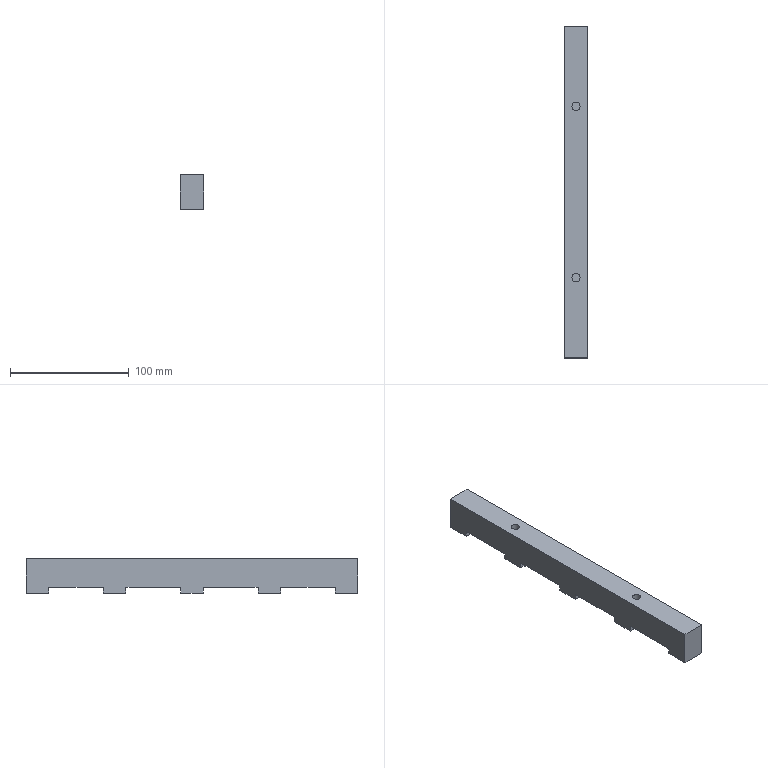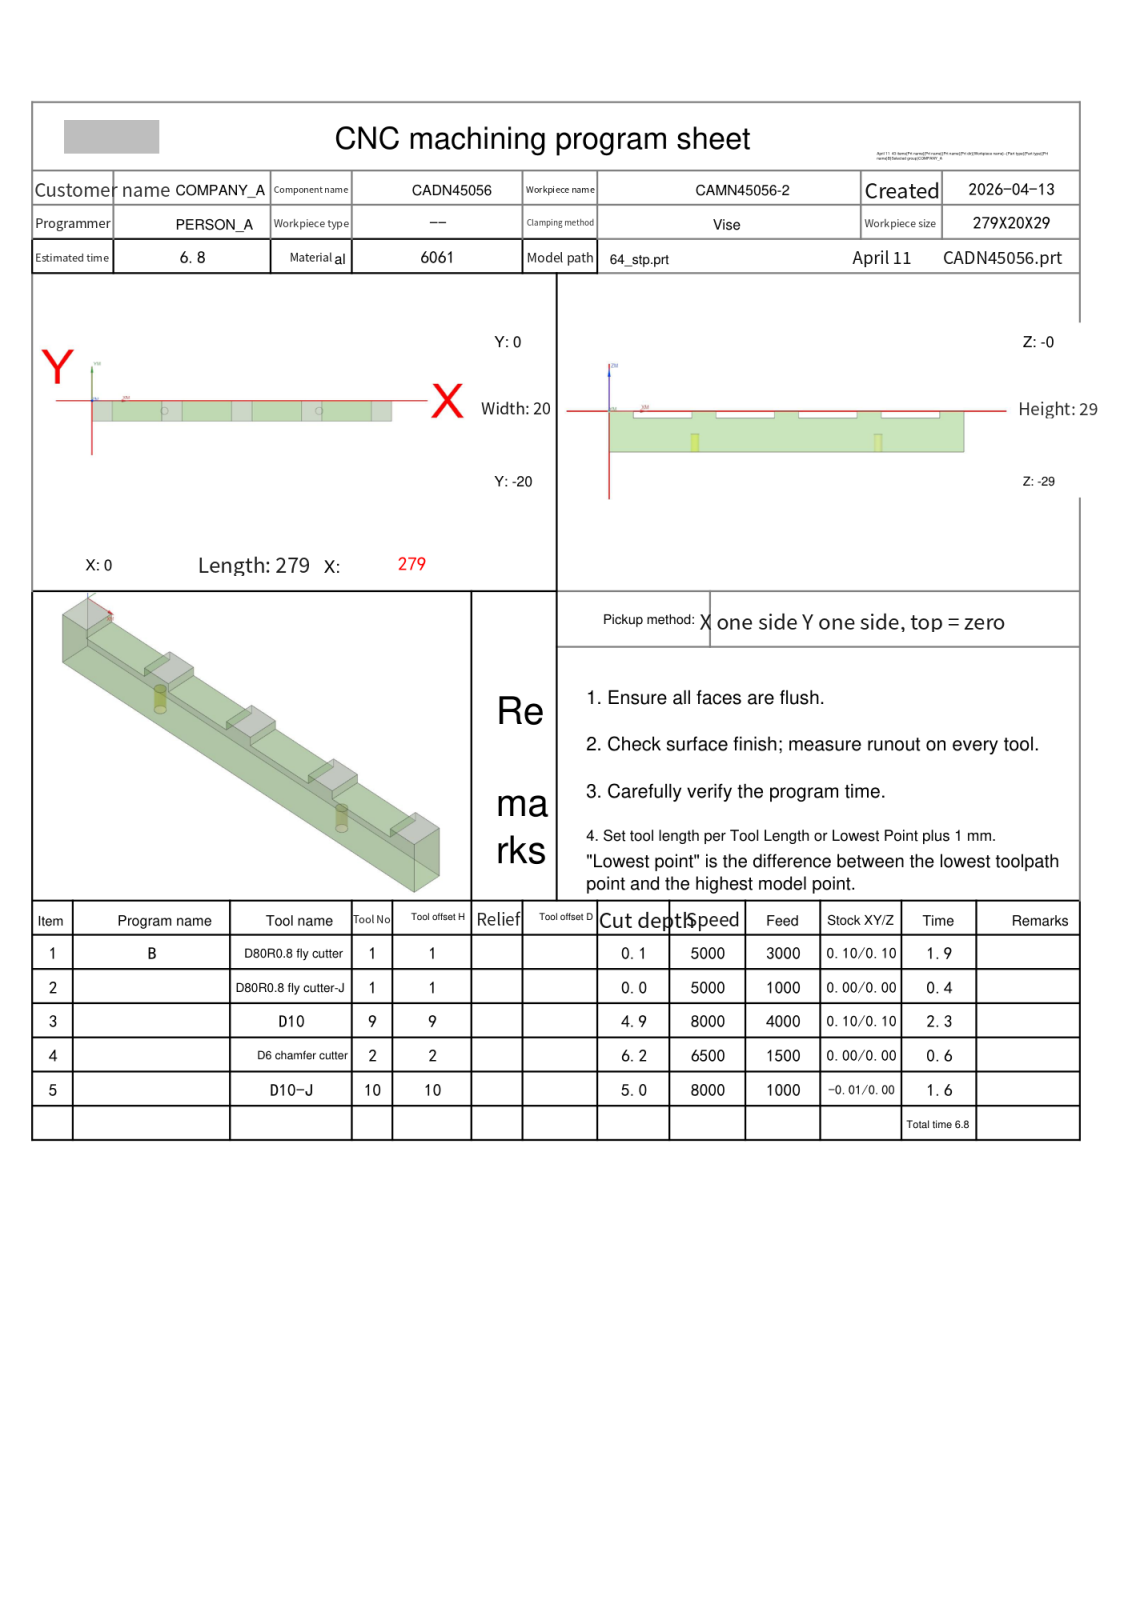NC program | NX | posted by the shop | part box 20 x 279 x 29 mm
Whole program:
%
O0001
(Machine time: 7.68 MIN)
(===Total Tool:4===)
(T1=D80R0.8 fly cutter D=80.  R=0.8  D-  H01 Z=0.    )
(T9=D10     D=10.  R=0.   D-  H09 Z=-4.9  )
(T2=D6 chamfer cutter   D=6.   R=0.   D-  H02 Z=-6.2  )
(T10=D10-J  D=10.  R=0.   D10 H10 Z=-5.   )
G80 G90 G17 G49 G40
G91 G28 Z0
M01
N1 T01 M06
(D80R0.8 fly cutter  D=80. R=0.8 H=01 ce=0.10 di=0.10)
G00 G90 G54 X-52.097 Y-10. M03 S5000
G43 H01 Z50.
M08
Z7.009
G01 Z5.009 F3000.
X-40.097
X319.097
X331.097
Z7.009
G00 X-52.097
Z6.518
G01 Z4.518
X-40.097
X319.097
X331.097
Z6.518
G00 X-52.097
Z6.027
G01 Z4.027
X-40.097
X319.097
X331.097
Z6.027
G00 X-52.097
Z5.536
G01 Z3.536
X-40.097
X319.097
X331.097
Z5.536
G00 Z50.
X-52.097
Z5.045
G01 Z3.045
X-40.097
X319.097
X331.097
Z5.045
G00 Z50.
X-52.097
Z4.555
G01 Z2.555
X-40.097
X319.097
X331.097
Z4.555
G00 Z50.
X-52.097
Z4.064
G01 Z2.064
X-40.097
X319.097
X331.097
Z4.064
G00 Z50.
X-52.097
Z3.573
G01 Z1.573
X-40.097
X319.097
X331.097
Z3.573
G00 Z50.
X-52.097
Z3.082
G01 Z1.082
X-40.097
X319.097
X331.097
Z3.082
G00 Z50.
X-52.097
Z2.591
G01 Z.591
X-40.097
X319.097
X331.097
Z2.591
G00 Z50.
X-52.097
Z2.1
G01 Z.1
X-40.097
X319.097
X331.097
Z2.1
G00 Z50.
G91 G28 Z0.0
M05
M09
G91 G28 Z0.0
M01
N2 T01 M06
(D80R0.8 fly cutter-J  D=80. R=0.8 H=01 ce=0.00 di=0.00)
G00 G90 G54 X-51.999 Y-10. M03 S5000
G43 H01 Z50.
M08
Z2.
G01 Z0.0 F1000.
X-39.999
X318.999
X330.999
Z2.
G00 Z50.
G91 G28 Z0.0
M05
M09
G91 G28 Z0.0
M01
N3 T09 M06
(D10  D=10. R=0. H=09 ce=0.10 di=0.10)
G00 G90 G54 X42. Y-28. M03 S8000
G43 H09 Z15.8
M08
Z.956
G01 Z-.544 F4000.
Y-24.9
X24.1
Y4.9
X59.9
Y-24.9
X45.035
G02 X44.203 Y-24.455 I0.0 J1.
G01 X39.797 Y-17.845
G03 X38.965 Y-17.4 I-.832 J-.555
G01 X32.596
G02 X31.6 Y-16.404 I.004 J1.
G01 Y-3.596
G02 X32.596 Y-2.6 I1. J-.004
G01 X51.404
G02 X52.4 Y-3.596 I-.004 J-1.
G01 Y-16.404
G02 X51.404 Y-17.4 I-1. J.004
G01 X44.664
G02 X43.957 Y-17.107 I0.0 J1.
G01 X40.043 Y-13.193
G03 X39.336 Y-12.9 I-.707 J-.707
G01 X37.096
G02 X36.1 Y-11.904 I.004 J1.
G01 Y-8.096
G02 X37.096 Y-7.1 I1. J-.004
G01 X46.904
G02 X47.9 Y-8.096 I-.004 J-1.
G01 Y-11.904
G02 X46.904 Y-12.9 I-1. J.004
G01 X42.
X41.5
Y-15.9
Z.956
G00 X42. Y-28.
Z.411
G01 Z-1.089
Y-24.9
X24.1
Y4.9
X59.9
Y-24.9
X45.035
G02 X44.203 Y-24.455 I0.0 J1.
G01 X39.797 Y-17.845
G03 X38.965 Y-17.4 I-.832 J-.555
G01 X32.596
G02 X31.6 Y-16.404 I.004 J1.
G01 Y-3.596
G02 X32.596 Y-2.6 I1. J-.004
G01 X51.404
G02 X52.4 Y-3.596 I-.004 J-1.
G01 Y-16.404
G02 X51.404 Y-17.4 I-1. J.004
G01 X44.664
G02 X43.957 Y-17.107 I0.0 J1.
G01 X40.043 Y-13.193
G03 X39.336 Y-12.9 I-.707 J-.707
G01 X37.096
G02 X36.1 Y-11.904 I.004 J1.
G01 Y-8.096
G02 X37.096 Y-7.1 I1. J-.004
G01 X46.904
G02 X47.9 Y-8.096 I-.004 J-1.
G01 Y-11.904
G02 X46.904 Y-12.9 I-1. J.004
G01 X42.
X41.5
Y-15.9
Z.411
G00 X42. Y-28.
Z-.133
G01 Z-1.633
Y-24.9
X24.1
Y4.9
X59.9
Y-24.9
X45.035
G02 X44.203 Y-24.455 I0.0 J1.
G01 X39.797 Y-17.845
G03 X38.965 Y-17.4 I-.832 J-.555
G01 X32.596
G02 X31.6 Y-16.404 I.004 J1.
G01 Y-3.596
G02 X32.596 Y-2.6 I1. J-.004
G01 X51.404
G02 X52.4 Y-3.596 I-.004 J-1.
G01 Y-16.404
G02 X51.404 Y-17.4 I-1. J.004
G01 X44.664
G02 X43.957 Y-17.107 I0.0 J1.
G01 X40.043 Y-13.193
G03 X39.336 Y-12.9 I-.707 J-.707
G01 X37.096
G02 X36.1 Y-11.904 I.004 J1.
G01 Y-8.096
G02 X37.096 Y-7.1 I1. J-.004
G01 X46.904
G02 X47.9 Y-8.096 I-.004 J-1.
G01 Y-11.904
G02 X46.904 Y-12.9 I-1. J.004
G01 X42.
X41.5
Y-15.9
Z-.133
G00 X42. Y-28.
Z-.678
G01 Z-2.178
Y-24.9
X24.1
Y4.9
X59.9
Y-24.9
X45.035
G02 X44.203 Y-24.455 I0.0 J1.
G01 X39.797 Y-17.845
G03 X38.965 Y-17.4 I-.832 J-.555
G01 X32.596
G02 X31.6 Y-16.404 I.004 J1.
G01 Y-3.596
G02 X32.596 Y-2.6 I1. J-.004
G01 X51.404
G02 X52.4 Y-3.596 I-.004 J-1.
G01 Y-16.404
G02 X51.404 Y-17.4 I-1. J.004
G01 X44.664
G02 X43.957 Y-17.107 I0.0 J1.
G01 X40.043 Y-13.193
G03 X39.336 Y-12.9 I-.707 J-.707
G01 X37.096
G02 X36.1 Y-11.904 I.004 J1.
G01 Y-8.096
G02 X37.096 Y-7.1 I1. J-.004
G01 X46.904
G02 X47.9 Y-8.096 I-.004 J-1.
G01 Y-11.904
G02 X46.904 Y-12.9 I-1. J.004
G01 X42.
X41.5
Y-15.9
Z-.678
G00 X42. Y-28.
Z-1.222
G01 Z-2.722
Y-24.9
X24.1
Y4.9
X59.9
Y-24.9
X45.035
G02 X44.203 Y-24.455 I0.0 J1.
G01 X39.797 Y-17.845
G03 X38.965 Y-17.4 I-.832 J-.555
G01 X32.596
G02 X31.6 Y-16.404 I.004 J1.
G01 Y-3.596
G02 X32.596 Y-2.6 I1. J-.004
G01 X51.404
G02 X52.4 Y-3.596 I-.004 J-1.
G01 Y-16.404
G02 X51.404 Y-17.4 I-1. J.004
G01 X44.664
G02 X43.957 Y-17.107 I0.0 J1.
G01 X40.043 Y-13.193
G03 X39.336 Y-12.9 I-.707 J-.707
G01 X37.096
G02 X36.1 Y-11.904 I.004 J1.
G01 Y-8.096
G02 X37.096 Y-7.1 I1. J-.004
G01 X46.904
G02 X47.9 Y-8.096 I-.004 J-1.
G01 Y-11.904
G02 X46.904 Y-12.9 I-1. J.004
G01 X42.
X41.5
Y-15.9
Z-1.222
G00 X42. Y-28.
Z-1.767
G01 Z-3.267
Y-24.9
X24.1
Y4.9
X59.9
Y-24.9
X45.035
G02 X44.203 Y-24.455 I0.0 J1.
G01 X39.797 Y-17.845
G03 X38.965 Y-17.4 I-.832 J-.555
G01 X32.596
G02 X31.6 Y-16.404 I.004 J1.
G01 Y-3.596
G02 X32.596 Y-2.6 I1. J-.004
G01 X51.404
G02 X52.4 Y-3.596 I-.004 J-1.
G01 Y-16.404
G02 X51.404 Y-17.4 I-1. J.004
G01 X44.664
G02 X43.957 Y-17.107 I0.0 J1.
G01 X40.043 Y-13.193
G03 X39.336 Y-12.9 I-.707 J-.707
G01 X37.096
G02 X36.1 Y-11.904 I.004 J1.
G01 Y-8.096
G02 X37.096 Y-7.1 I1. J-.004
G01 X46.904
G02 X47.9 Y-8.096 I-.004 J-1.
G01 Y-11.904
G02 X46.904 Y-12.9 I-1. J.004
G01 X42.
X41.5
Y-15.9
Z-1.767
G00 X42. Y-28.
Z-2.311
G01 Z-3.811
Y-24.9
X24.1
Y4.9
X59.9
Y-24.9
X45.035
G02 X44.203 Y-24.455 I0.0 J1.
G01 X39.797 Y-17.845
G03 X38.965 Y-17.4 I-.832 J-.555
G01 X32.596
G02 X31.6 Y-16.404 I.004 J1.
G01 Y-3.596
G02 X32.596 Y-2.6 I1. J-.004
G01 X51.404
G02 X52.4 Y-3.596 I-.004 J-1.
G01 Y-16.404
G02 X51.404 Y-17.4 I-1. J.004
G01 X44.664
G02 X43.957 Y-17.107 I0.0 J1.
G01 X40.043 Y-13.193
G03 X39.336 Y-12.9 I-.707 J-.707
G01 X37.096
G02 X36.1 Y-11.904 I.004 J1.
G01 Y-8.096
G02 X37.096 Y-7.1 I1. J-.004
G01 X46.904
G02 X47.9 Y-8.096 I-.004 J-1.
G01 Y-11.904
G02 X46.904 Y-12.9 I-1. J.004
G01 X42.
X41.5
Y-15.9
Z-2.311
G00 X42. Y-28.
Z-2.856
G01 Z-4.356
Y-24.9
X24.1
Y4.9
X59.9
Y-24.9
X45.035
G02 X44.203 Y-24.455 I0.0 J1.
G01 X39.797 Y-17.845
G03 X38.965 Y-17.4 I-.832 J-.555
G01 X32.596
G02 X31.6 Y-16.404 I.004 J1.
G01 Y-3.596
G02 X32.596 Y-2.6 I1. J-.004
G01 X51.404
G02 X52.4 Y-3.596 I-.004 J-1.
G01 Y-16.404
G02 X51.404 Y-17.4 I-1. J.004
G01 X44.664
G02 X43.957 Y-17.107 I0.0 J1.
G01 X40.043 Y-13.193
G03 X39.336 Y-12.9 I-.707 J-.707
G01 X37.096
G02 X36.1 Y-11.904 I.004 J1.
G01 Y-8.096
G02 X37.096 Y-7.1 I1. J-.004
G01 X46.904
G02 X47.9 Y-8.096 I-.004 J-1.
G01 Y-11.904
G02 X46.904 Y-12.9 I-1. J.004
G01 X42.
X41.5
Y-15.9
Z-2.856
G00 X42. Y-28.
Z-3.4
G01 Z-4.9
Y-24.9
X24.1
Y4.9
X59.9
Y-24.9
X45.035
G02 X44.203 Y-24.455 I0.0 J1.
G01 X39.797 Y-17.845
G03 X38.965 Y-17.4 I-.832 J-.555
G01 X32.596
G02 X31.6 Y-16.404 I.004 J1.
G01 Y-3.596
G02 X32.596 Y-2.6 I1. J-.004
G01 X51.404
G02 X52.4 Y-3.596 I-.004 J-1.
G01 Y-16.404
G02 X51.404 Y-17.4 I-1. J.004
G01 X44.664
G02 X43.957 Y-17.107 I0.0 J1.
G01 X40.043 Y-13.193
G03 X39.336 Y-12.9 I-.707 J-.707
G01 X37.096
G02 X36.1 Y-11.904 I.004 J1.
G01 Y-8.096
G02 X37.096 Y-7.1 I1. J-.004
G01 X46.904
G02 X47.9 Y-8.096 I-.004 J-1.
G01 Y-11.904
G02 X46.904 Y-12.9 I-1. J.004
G01 X42.
X41.5
Y-15.9
Z-3.4
G00 Z15.8
X107. Y-28.
Z.956
G01 Z-.544
Y-24.9
X89.1
Y4.9
X124.9
Y-24.9
X110.035
G02 X109.203 Y-24.455 I0.0 J1.
G01 X104.797 Y-17.845
G03 X103.965 Y-17.4 I-.832 J-.555
G01 X97.596
G02 X96.6 Y-16.404 I.004 J1.
G01 Y-3.596
G02 X97.596 Y-2.6 I1. J-.004
G01 X116.404
G02 X117.4 Y-3.596 I-.004 J-1.
G01 Y-16.404
G02 X116.404 Y-17.4 I-1. J.004
G01 X109.664
G02 X108.957 Y-17.107 I0.0 J1.
G01 X105.043 Y-13.193
G03 X104.336 Y-12.9 I-.707 J-.707
G01 X102.096
G02 X101.1 Y-11.904 I.004 J1.
G01 Y-8.096
G02 X102.096 Y-7.1 I1. J-.004
G01 X111.904
G02 X112.9 Y-8.096 I-.004 J-1.
G01 Y-11.904
G02 X111.904 Y-12.9 I-1. J.004
G01 X107.
X106.5
Y-15.9
Z.956
G00 X107. Y-28.
Z.411
G01 Z-1.089
Y-24.9
X89.1
Y4.9
X124.9
Y-24.9
X110.035
G02 X109.203 Y-24.455 I0.0 J1.
G01 X104.797 Y-17.845
G03 X103.965 Y-17.4 I-.832 J-.555
G01 X97.596
G02 X96.6 Y-16.404 I.004 J1.
G01 Y-3.596
G02 X97.596 Y-2.6 I1. J-.004
G01 X116.404
G02 X117.4 Y-3.596 I-.004 J-1.
G01 Y-16.404
G02 X116.404 Y-17.4 I-1. J.004
G01 X109.664
G02 X108.957 Y-17.107 I0.0 J1.
G01 X105.043 Y-13.193
G03 X104.336 Y-12.9 I-.707 J-.707
G01 X102.096
G02 X101.1 Y-11.904 I.004 J1.
G01 Y-8.096
G02 X102.096 Y-7.1 I1. J-.004
G01 X111.904
G02 X112.9 Y-8.096 I-.004 J-1.
G01 Y-11.904
G02 X111.904 Y-12.9 I-1. J.004
G01 X107.
X106.5
Y-15.9
Z.411
G00 X107. Y-28.
Z-.133
G01 Z-1.633
Y-24.9
X89.1
Y4.9
X124.9
Y-24.9
X110.035
G02 X109.203 Y-24.455 I0.0 J1.
G01 X104.797 Y-17.845
G03 X103.965 Y-17.4 I-.832 J-.555
G01 X97.596
G02 X96.6 Y-16.404 I.004 J1.
G01 Y-3.596
G02 X97.596 Y-2.6 I1. J-.004
G01 X116.404
G02 X117.4 Y-3.596 I-.004 J-1.
G01 Y-16.404
G02 X116.404 Y-17.4 I-1. J.004
G01 X109.664
G02 X108.957 Y-17.107 I0.0 J1.
G01 X105.043 Y-13.193
G03 X104.336 Y-12.9 I-.707 J-.707
G01 X102.096
G02 X101.1 Y-11.904 I.004 J1.
G01 Y-8.096
G02 X102.096 Y-7.1 I1. J-.004
G01 X111.904
G02 X112.9 Y-8.096 I-.004 J-1.
G01 Y-11.904
G02 X111.904 Y-12.9 I-1. J.004
G01 X107.
X106.5
Y-15.9
Z-.133
G00 X107. Y-28.
Z-.678
G01 Z-2.178
Y-24.9
X89.1
Y4.9
X124.9
Y-24.9
X110.035
G02 X109.203 Y-24.455 I0.0 J1.
G01 X104.797 Y-17.845
G03 X103.965 Y-17.4 I-.832 J-.555
G01 X97.596
G02 X96.6 Y-16.404 I.004 J1.
G01 Y-3.596
G02 X97.596 Y-2.6 I1. J-.004
G01 X116.404
G02 X117.4 Y-3.596 I-.004 J-1.
G01 Y-16.404
G02 X116.404 Y-17.4 I-1. J.004
G01 X109.664
G02 X108.957 Y-17.107 I0.0 J1.
G01 X105.043 Y-13.193
G03 X104.336 Y-12.9 I-.707 J-.707
G01 X102.096
G02 X101.1 Y-11.904 I.004 J1.
G01 Y-8.096
G02 X102.096 Y-7.1 I1. J-.004
G01 X111.904
G02 X112.9 Y-8.096 I-.004 J-1.
G01 Y-11.904
G02 X111.904 Y-12.9 I-1. J.004
G01 X107.
X106.5
Y-15.9
Z-.678
G00 X107. Y-28.
Z-1.222
G01 Z-2.722
Y-24.9
X89.1
Y4.9
X124.9
Y-24.9
X110.035
G02 X109.203 Y-24.455 I0.0 J1.
G01 X104.797 Y-17.845
G03 X103.965 Y-17.4 I-.832 J-.555
G01 X97.596
G02 X96.6 Y-16.404 I.004 J1.
G01 Y-3.596
G02 X97.596 Y-2.6 I1. J-.004
G01 X116.404
G02 X117.4 Y-3.596 I-.004 J-1.
G01 Y-16.404
G02 X116.404 Y-17.4 I-1. J.004
G01 X109.664
G02 X108.957 Y-17.107 I0.0 J1.
G01 X105.043 Y-13.193
G03 X104.336 Y-12.9 I-.707 J-.707
G01 X102.096
G02 X101.1 Y-11.904 I.004 J1.
G01 Y-8.096
G02 X102.096 Y-7.1 I1. J-.004
G01 X111.904
G02 X112.9 Y-8.096 I-.004 J-1.
G01 Y-11.904
G02 X111.904 Y-12.9 I-1. J.004
G01 X107.
X106.5
Y-15.9
Z-1.222
G00 X107. Y-28.
Z-1.767
G01 Z-3.267
Y-24.9
X89.1
Y4.9
X124.9
Y-24.9
X110.035
G02 X109.203 Y-24.455 I0.0 J1.
G01 X104.797 Y-17.845
G03 X103.965 Y-17.4 I-.832 J-.555
G01 X97.596
G02 X96.6 Y-16.404 I.004 J1.
G01 Y-3.596
G02 X97.596 Y-2.6 I1. J-.004
G01 X116.404
G02 X117.4 Y-3.596 I-.004 J-1.
G01 Y-16.404
G02 X116.404 Y-17.4 I-1. J.004
G01 X109.664
G02 X108.957 Y-17.107 I0.0 J1.
G01 X105.043 Y-13.193
G03 X104.336 Y-12.9 I-.707 J-.707
G01 X102.096
G02 X101.1 Y-11.904 I.004 J1.
G01 Y-8.096
G02 X102.096 Y-7.1 I1. J-.004
G01 X111.904
G02 X112.9 Y-8.096 I-.004 J-1.
G01 Y-11.904
G02 X111.904 Y-12.9 I-1. J.004
G01 X107.
X106.5
Y-15.9
Z-1.767
G00 X107. Y-28.
Z-2.311
G01 Z-3.811
Y-24.9
X89.1
Y4.9
X124.9
Y-24.9
X110.035
G02 X109.203 Y-24.455 I0.0 J1.
G01 X104.797 Y-17.845
G03 X103.965 Y-17.4 I-.832 J-.555
G01 X97.596
G02 X96.6 Y-16.404 I.004 J1.
G01 Y-3.596
G02 X97.596 Y-2.6 I1. J-.004
G01 X116.404
G02 X117.4 Y-3.596 I-.004 J-1.
G01 Y-16.404
G02 X116.404 Y-17.4 I-1. J.004
G01 X109.664
G02 X108.957 Y-17.107 I0.0 J1.
G01 X105.043 Y-13.193
G03 X104.336 Y-12.9 I-.707 J-.707
G01 X102.096
G02 X101.1 Y-11.904 I.004 J1.
G01 Y-8.096
G02 X102.096 Y-7.1 I1. J-.004
G01 X111.904
G02 X112.9 Y-8.096 I-.004 J-1.
G01 Y-11.904
G02 X111.904 Y-12.9 I-1. J.004
G01 X107.
X106.5
Y-15.9
Z-2.311
G00 X107. Y-28.
Z-2.856
G01 Z-4.356
Y-24.9
X89.1
Y4.9
X124.9
Y-24.9
X110.035
G02 X109.203 Y-24.455 I0.0 J1.
G01 X104.797 Y-17.845
G03 X103.965 Y-17.4 I-.832 J-.555
G01 X97.596
G02 X96.6 Y-16.404 I.004 J1.
G01 Y-3.596
G02 X97.596 Y-2.6 I1. J-.004
G01 X116.404
G02 X117.4 Y-3.596 I-.004 J-1.
G01 Y-16.404
G02 X116.404 Y-17.4 I-1. J.004
G01 X109.664
G02 X108.957 Y-17.107 I0.0 J1.
G01 X105.043 Y-13.193
G03 X104.336 Y-12.9 I-.707 J-.707
G01 X102.096
G02 X101.1 Y-11.904 I.004 J1.
G01 Y-8.096
G02 X102.096 Y-7.1 I1. J-.004
G01 X111.904
G02 X112.9 Y-8.096 I-.004 J-1.
G01 Y-11.904
G02 X111.904 Y-12.9 I-1. J.004
G01 X107.
X106.5
Y-15.9
Z-2.856
G00 X107. Y-28.
Z-3.4
G01 Z-4.9
Y-24.9
X89.1
Y4.9
X124.9
Y-24.9
X110.035
G02 X109.203 Y-24.455 I0.0 J1.
G01 X104.797 Y-17.845
G03 X103.965 Y-17.4 I-.832 J-.555
G01 X97.596
G02 X96.6 Y-16.404 I.004 J1.
G01 Y-3.596
G02 X97.596 Y-2.6 I1. J-.004
G01 X116.404
G02 X117.4 Y-3.596 I-.004 J-1.
G01 Y-16.404
G02 X116.404 Y-17.4 I-1. J.004
G01 X109.664
G02 X108.957 Y-17.107 I0.0 J1.
G01 X105.043 Y-13.193
G03 X104.336 Y-12.9 I-.707 J-.707
G01 X102.096
G02 X101.1 Y-11.904 I.004 J1.
G01 Y-8.096
G02 X102.096 Y-7.1 I1. J-.004
G01 X111.904
G02 X112.9 Y-8.096 I-.004 J-1.
G01 Y-11.904
G02 X111.904 Y-12.9 I-1. J.004
G01 X107.
X106.5
Y-15.9
Z-3.4
G00 Z15.8
X172. Y-28.
Z.956
G01 Z-.544
Y-24.9
X154.1
Y4.9
X189.9
Y-24.9
X175.035
G02 X174.203 Y-24.455 I0.0 J1.
G01 X169.797 Y-17.845
G03 X168.965 Y-17.4 I-.832 J-.555
G01 X162.596
G02 X161.6 Y-16.404 I.004 J1.
G01 Y-3.596
G02 X162.596 Y-2.6 I1. J-.004
G01 X181.404
G02 X182.4 Y-3.596 I-.004 J-1.
G01 Y-16.404
G02 X181.404 Y-17.4 I-1. J.004
G01 X174.664
G02 X173.957 Y-17.107 I0.0 J1.
G01 X170.043 Y-13.193
G03 X169.336 Y-12.9 I-.707 J-.707
G01 X167.096
G02 X166.1 Y-11.904 I.004 J1.
G01 Y-8.096
G02 X167.096 Y-7.1 I1. J-.004
G01 X176.904
G02 X177.9 Y-8.096 I-.004 J-1.
G01 Y-11.904
G02 X176.904 Y-12.9 I-1. J.004
G01 X172.
X171.5
Y-15.9
Z.956
G00 X172. Y-28.
Z.411
G01 Z-1.089
Y-24.9
X154.1
Y4.9
X189.9
Y-24.9
X175.035
G02 X174.203 Y-24.455 I0.0 J1.
G01 X169.797 Y-17.845
G03 X168.965 Y-17.4 I-.832 J-.555
G01 X162.596
G02 X161.6 Y-16.404 I.004 J1.
G01 Y-3.596
G02 X162.596 Y-2.6 I1. J-.004
G01 X181.404
G02 X182.4 Y-3.596 I-.004 J-1.
G01 Y-16.404
G02 X181.404 Y-17.4 I-1. J.004
G01 X174.664
G02 X173.957 Y-17.107 I0.0 J1.
G01 X170.043 Y-13.193
G03 X169.336 Y-12.9 I-.707 J-.707
G01 X167.096
G02 X166.1 Y-11.904 I.004 J1.
G01 Y-8.096
G02 X167.096 Y-7.1 I1. J-.004
G01 X176.904
G02 X177.9 Y-8.096 I-.004 J-1.
G01 Y-11.904
G02 X176.904 Y-12.9 I-1. J.004
G01 X172.
X171.5
Y-15.9
Z.411
G00 X172. Y-28.
Z-.133
G01 Z-1.633
Y-24.9
X154.1
Y4.9
X189.9
Y-24.9
X175.035
G02 X174.203 Y-24.455 I0.0 J1.
G01 X169.797 Y-17.845
G03 X168.965 Y-17.4 I-.832 J-.555
G01 X162.596
G02 X161.6 Y-16.404 I.004 J1.
G01 Y-3.596
G02 X162.596 Y-2.6 I1. J-.004
G01 X181.404
G02 X182.4 Y-3.596 I-.004 J-1.
G01 Y-16.404
G02 X181.404 Y-17.4 I-1. J.004
G01 X174.664
G02 X173.957 Y-17.107 I0.0 J1.
G01 X170.043 Y-13.193
G03 X169.336 Y-12.9 I-.707 J-.707
G01 X167.096
G02 X166.1 Y-11.904 I.004 J1.
G01 Y-8.096
G02 X167.096 Y-7.1 I1. J-.004
G01 X176.904
G02 X177.9 Y-8.096 I-.004 J-1.
G01 Y-11.904
G02 X176.904 Y-12.9 I-1. J.004
G01 X172.
X171.5
Y-15.9
Z-.133
G00 X172. Y-28.
Z-.678
G01 Z-2.178
Y-24.9
X154.1
Y4.9
X189.9
Y-24.9
X175.035
G02 X174.203 Y-24.455 I0.0 J1.
G01 X169.797 Y-17.845
G03 X168.965 Y-17.4 I-.832 J-.555
G01 X162.596
G02 X161.6 Y-16.404 I.004 J1.
G01 Y-3.596
G02 X162.596 Y-2.6 I1. J-.004
G01 X181.404
G02 X182.4 Y-3.596 I-.004 J-1.
G01 Y-16.404
G02 X181.404 Y-17.4 I-1. J.004
G01 X174.664
G02 X173.957 Y-17.107 I0.0 J1.
G01 X170.043 Y-13.193
G03 X169.336 Y-12.9 I-.707 J-.707
G01 X167.096
G02 X166.1 Y-11.904 I.004 J1.
G01 Y-8.096
G02 X167.096 Y-7.1 I1. J-.004
G01 X176.904
G02 X177.9 Y-8.096 I-.004 J-1.
G01 Y-11.904
G02 X176.904 Y-12.9 I-1. J.004
G01 X172.
X171.5
Y-15.9
Z-.678
G00 X172. Y-28.
Z-1.222
G01 Z-2.722
Y-24.9
X154.1
Y4.9
X189.9
Y-24.9
X175.035
G02 X174.203 Y-24.455 I0.0 J1.
G01 X169.797 Y-17.845
G03 X168.965 Y-17.4 I-.832 J-.555
G01 X162.596
G02 X161.6 Y-16.404 I.004 J1.
G01 Y-3.596
G02 X162.596 Y-2.6 I1. J-.004
G01 X181.404
G02 X182.4 Y-3.596 I-.004 J-1.
G01 Y-16.404
G02 X181.404 Y-17.4 I-1. J.004
G01 X174.664
G02 X173.957 Y-17.107 I0.0 J1.
G01 X170.043 Y-13.193
G03 X169.336 Y-12.9 I-.707 J-.707
G01 X167.096
G02 X166.1 Y-11.904 I.004 J1.
G01 Y-8.096
G02 X167.096 Y-7.1 I1. J-.004
G01 X176.904
G02 X177.9 Y-8.096 I-.004 J-1.
G01 Y-11.904
G02 X176.904 Y-12.9 I-1. J.004
G01 X172.
X171.5
Y-15.9
Z-1.222
G00 X172. Y-28.
Z-1.767
G01 Z-3.267
Y-24.9
X154.1
Y4.9
X189.9
Y-24.9
X175.035
G02 X174.203 Y-24.455 I0.0 J1.
G01 X169.797 Y-17.845
G03 X168.965 Y-17.4 I-.832 J-.555
G01 X162.596
G02 X161.6 Y-16.404 I.004 J1.
G01 Y-3.596
G02 X162.596 Y-2.6 I1. J-.004
G01 X181.404
G02 X182.4 Y-3.596 I-.004 J-1.
G01 Y-16.404
G02 X181.404 Y-17.4 I-1. J.004
G01 X174.664
G02 X173.957 Y-17.107 I0.0 J1.
G01 X170.043 Y-13.193
G03 X169.336 Y-12.9 I-.707 J-.707
G01 X167.096
G02 X166.1 Y-11.904 I.004 J1.
G01 Y-8.096
G02 X167.096 Y-7.1 I1. J-.004
G01 X176.904
G02 X177.9 Y-8.096 I-.004 J-1.
G01 Y-11.904
G02 X176.904 Y-12.9 I-1. J.004
G01 X172.
X171.5
Y-15.9
Z-1.767
G00 X172. Y-28.
Z-2.311
G01 Z-3.811
Y-24.9
X154.1
Y4.9
X189.9
Y-24.9
X175.035
G02 X174.203 Y-24.455 I0.0 J1.
G01 X169.797 Y-17.845
G03 X168.965 Y-17.4 I-.832 J-.555
G01 X162.596
G02 X161.6 Y-16.404 I.004 J1.
G01 Y-3.596
G02 X162.596 Y-2.6 I1. J-.004
G01 X181.404
G02 X182.4 Y-3.596 I-.004 J-1.
G01 Y-16.404
G02 X181.404 Y-17.4 I-1. J.004
G01 X174.664
G02 X173.957 Y-17.107 I0.0 J1.
G01 X170.043 Y-13.193
G03 X169.336 Y-12.9 I-.707 J-.707
G01 X167.096
G02 X166.1 Y-11.904 I.004 J1.
G01 Y-8.096
G02 X167.096 Y-7.1 I1. J-.004
G01 X176.904
G02 X177.9 Y-8.096 I-.004 J-1.
G01 Y-11.904
G02 X176.904 Y-12.9 I-1. J.004
G01 X172.
X171.5
Y-15.9
Z-2.311
G00 X172. Y-28.
Z-2.856
G01 Z-4.356
Y-24.9
X154.1
Y4.9
X189.9
Y-24.9
X175.035
G02 X174.203 Y-24.455 I0.0 J1.
G01 X169.797 Y-17.845
G03 X168.965 Y-17.4 I-.832 J-.555
G01 X162.596
G02 X161.6 Y-16.404 I.004 J1.
G01 Y-3.596
G02 X162.596 Y-2.6 I1. J-.004
G01 X181.404
G02 X182.4 Y-3.596 I-.004 J-1.
G01 Y-16.404
G02 X181.404 Y-17.4 I-1. J.004
G01 X174.664
G02 X173.957 Y-17.107 I0.0 J1.
G01 X170.043 Y-13.193
G03 X169.336 Y-12.9 I-.707 J-.707
G01 X167.096
G02 X166.1 Y-11.904 I.004 J1.
G01 Y-8.096
G02 X167.096 Y-7.1 I1. J-.004
G01 X176.904
G02 X177.9 Y-8.096 I-.004 J-1.
G01 Y-11.904
G02 X176.904 Y-12.9 I-1. J.004
G01 X172.
X171.5
Y-15.9
Z-2.856
G00 X172. Y-28.
Z-3.4
G01 Z-4.9
Y-24.9
X154.1
Y4.9
X189.9
Y-24.9
X175.035
G02 X174.203 Y-24.455 I0.0 J1.
G01 X169.797 Y-17.845
G03 X168.965 Y-17.4 I-.832 J-.555
G01 X162.596
G02 X161.6 Y-16.404 I.004 J1.
G01 Y-3.596
G02 X162.596 Y-2.6 I1. J-.004
G01 X181.404
G02 X182.4 Y-3.596 I-.004 J-1.
G01 Y-16.404
G02 X181.404 Y-17.4 I-1. J.004
G01 X174.664
G02 X173.957 Y-17.107 I0.0 J1.
G01 X170.043 Y-13.193
G03 X169.336 Y-12.9 I-.707 J-.707
G01 X167.096
G02 X166.1 Y-11.904 I.004 J1.
G01 Y-8.096
G02 X167.096 Y-7.1 I1. J-.004
G01 X176.904
G02 X177.9 Y-8.096 I-.004 J-1.
G01 Y-11.904
G02 X176.904 Y-12.9 I-1. J.004
G01 X172.
X171.5
Y-15.9
Z-3.4
G00 Z15.8
X237. Y-28.
Z.956
G01 Z-.544
Y-24.9
X219.1
Y4.9
X254.9
Y-24.9
X240.035
G02 X239.203 Y-24.455 I0.0 J1.
G01 X234.797 Y-17.845
G03 X233.965 Y-17.4 I-.832 J-.555
G01 X227.596
G02 X226.6 Y-16.404 I.004 J1.
G01 Y-3.596
G02 X227.596 Y-2.6 I1. J-.004
G01 X246.404
G02 X247.4 Y-3.596 I-.004 J-1.
G01 Y-16.404
G02 X246.404 Y-17.4 I-1. J.004
G01 X239.664
G02 X238.957 Y-17.107 I0.0 J1.
G01 X235.043 Y-13.193
G03 X234.336 Y-12.9 I-.707 J-.707
G01 X232.096
G02 X231.1 Y-11.904 I.004 J1.
G01 Y-8.096
G02 X232.096 Y-7.1 I1. J-.004
G01 X241.904
G02 X242.9 Y-8.096 I-.004 J-1.
G01 Y-11.904
G02 X241.904 Y-12.9 I-1. J.004
G01 X237.
X236.5
Y-15.9
Z.956
G00 X237. Y-28.
Z.411
G01 Z-1.089
Y-24.9
X219.1
Y4.9
X254.9
Y-24.9
X240.035
G02 X239.203 Y-24.455 I0.0 J1.
G01 X234.797 Y-17.845
G03 X233.965 Y-17.4 I-.832 J-.555
G01 X227.596
G02 X226.6 Y-16.404 I.004 J1.
G01 Y-3.596
G02 X227.596 Y-2.6 I1. J-.004
G01 X246.404
G02 X247.4 Y-3.596 I-.004 J-1.
G01 Y-16.404
G02 X246.404 Y-17.4 I-1. J.004
G01 X239.664
G02 X238.957 Y-17.107 I0.0 J1.
G01 X235.043 Y-13.193
G03 X234.336 Y-12.9 I-.707 J-.707
G01 X232.096
G02 X231.1 Y-11.904 I.004 J1.
G01 Y-8.096
G02 X232.096 Y-7.1 I1. J-.004
G01 X241.904
G02 X242.9 Y-8.096 I-.004 J-1.
G01 Y-11.904
G02 X241.904 Y-12.9 I-1. J.004
G01 X237.
X236.5
Y-15.9
Z.411
G00 X237. Y-28.
Z-.133
G01 Z-1.633
Y-24.9
X219.1
Y4.9
X254.9
Y-24.9
X240.035
G02 X239.203 Y-24.455 I0.0 J1.
G01 X234.797 Y-17.845
G03 X233.965 Y-17.4 I-.832 J-.555
G01 X227.596
G02 X226.6 Y-16.404 I.004 J1.
G01 Y-3.596
G02 X227.596 Y-2.6 I1. J-.004
G01 X246.404
G02 X247.4 Y-3.596 I-.004 J-1.
G01 Y-16.404
G02 X246.404 Y-17.4 I-1. J.004
G01 X239.664
G02 X238.957 Y-17.107 I0.0 J1.
G01 X235.043 Y-13.193
G03 X234.336 Y-12.9 I-.707 J-.707
G01 X232.096
G02 X231.1 Y-11.904 I.004 J1.
G01 Y-8.096
G02 X232.096 Y-7.1 I1. J-.004
G01 X241.904
G02 X242.9 Y-8.096 I-.004 J-1.
G01 Y-11.904
G02 X241.904 Y-12.9 I-1. J.004
G01 X237.
X236.5
Y-15.9
Z-.133
G00 X237. Y-28.
Z-.678
G01 Z-2.178
Y-24.9
X219.1
Y4.9
X254.9
Y-24.9
X240.035
G02 X239.203 Y-24.455 I0.0 J1.
G01 X234.797 Y-17.845
G03 X233.965 Y-17.4 I-.832 J-.555
G01 X227.596
G02 X226.6 Y-16.404 I.004 J1.
G01 Y-3.596
G02 X227.596 Y-2.6 I1. J-.004
G01 X246.404
G02 X247.4 Y-3.596 I-.004 J-1.
G01 Y-16.404
G02 X246.404 Y-17.4 I-1. J.004
G01 X239.664
G02 X238.957 Y-17.107 I0.0 J1.
G01 X235.043 Y-13.193
G03 X234.336 Y-12.9 I-.707 J-.707
G01 X232.096
G02 X231.1 Y-11.904 I.004 J1.
G01 Y-8.096
G02 X232.096 Y-7.1 I1. J-.004
G01 X241.904
G02 X242.9 Y-8.096 I-.004 J-1.
G01 Y-11.904
G02 X241.904 Y-12.9 I-1. J.004
G01 X237.
X236.5
Y-15.9
Z-.678
G00 X237. Y-28.
Z-1.222
G01 Z-2.722
Y-24.9
X219.1
Y4.9
X254.9
Y-24.9
X240.035
G02 X239.203 Y-24.455 I0.0 J1.
G01 X234.797 Y-17.845
G03 X233.965 Y-17.4 I-.832 J-.555
G01 X227.596
G02 X226.6 Y-16.404 I.004 J1.
G01 Y-3.596
G02 X227.596 Y-2.6 I1. J-.004
G01 X246.404
G02 X247.4 Y-3.596 I-.004 J-1.
G01 Y-16.404
G02 X246.404 Y-17.4 I-1. J.004
G01 X239.664
G02 X238.957 Y-17.107 I0.0 J1.
G01 X235.043 Y-13.193
G03 X234.336 Y-12.9 I-.707 J-.707
G01 X232.096
G02 X231.1 Y-11.904 I.004 J1.
G01 Y-8.096
G02 X232.096 Y-7.1 I1. J-.004
G01 X241.904
G02 X242.9 Y-8.096 I-.004 J-1.
G01 Y-11.904
G02 X241.904 Y-12.9 I-1. J.004
G01 X237.
X236.5
Y-15.9
Z-1.222
G00 X237. Y-28.
Z-1.767
G01 Z-3.267
Y-24.9
X219.1
Y4.9
X254.9
Y-24.9
X240.035
G02 X239.203 Y-24.455 I0.0 J1.
G01 X234.797 Y-17.845
G03 X233.965 Y-17.4 I-.832 J-.555
G01 X227.596
G02 X226.6 Y-16.404 I.004 J1.
G01 Y-3.596
G02 X227.596 Y-2.6 I1. J-.004
G01 X246.404
G02 X247.4 Y-3.596 I-.004 J-1.
G01 Y-16.404
G02 X246.404 Y-17.4 I-1. J.004
G01 X239.664
G02 X238.957 Y-17.107 I0.0 J1.
G01 X235.043 Y-13.193
G03 X234.336 Y-12.9 I-.707 J-.707
G01 X232.096
G02 X231.1 Y-11.904 I.004 J1.
G01 Y-8.096
G02 X232.096 Y-7.1 I1. J-.004
G01 X241.904
G02 X242.9 Y-8.096 I-.004 J-1.
G01 Y-11.904
G02 X241.904 Y-12.9 I-1. J.004
G01 X237.
X236.5
Y-15.9
Z-1.767
G00 X237. Y-28.
Z-2.311
G01 Z-3.811
Y-24.9
X219.1
Y4.9
X254.9
Y-24.9
X240.035
G02 X239.203 Y-24.455 I0.0 J1.
G01 X234.797 Y-17.845
G03 X233.965 Y-17.4 I-.832 J-.555
G01 X227.596
G02 X226.6 Y-16.404 I.004 J1.
G01 Y-3.596
G02 X227.596 Y-2.6 I1. J-.004
G01 X246.404
G02 X247.4 Y-3.596 I-.004 J-1.
G01 Y-16.404
G02 X246.404 Y-17.4 I-1. J.004
G01 X239.664
G02 X238.957 Y-17.107 I0.0 J1.
G01 X235.043 Y-13.193
G03 X234.336 Y-12.9 I-.707 J-.707
G01 X232.096
G02 X231.1 Y-11.904 I.004 J1.
G01 Y-8.096
G02 X232.096 Y-7.1 I1. J-.004
G01 X241.904
G02 X242.9 Y-8.096 I-.004 J-1.
G01 Y-11.904
G02 X241.904 Y-12.9 I-1. J.004
G01 X237.
X236.5
Y-15.9
Z-2.311
G00 X237. Y-28.
Z-2.856
G01 Z-4.356
Y-24.9
X219.1
Y4.9
X254.9
Y-24.9
X240.035
G02 X239.203 Y-24.455 I0.0 J1.
G01 X234.797 Y-17.845
G03 X233.965 Y-17.4 I-.832 J-.555
G01 X227.596
G02 X226.6 Y-16.404 I.004 J1.
G01 Y-3.596
G02 X227.596 Y-2.6 I1. J-.004
G01 X246.404
G02 X247.4 Y-3.596 I-.004 J-1.
G01 Y-16.404
G02 X246.404 Y-17.4 I-1. J.004
G01 X239.664
G02 X238.957 Y-17.107 I0.0 J1.
G01 X235.043 Y-13.193
G03 X234.336 Y-12.9 I-.707 J-.707
G01 X232.096
G02 X231.1 Y-11.904 I.004 J1.
G01 Y-8.096
G02 X232.096 Y-7.1 I1. J-.004
G01 X241.904
G02 X242.9 Y-8.096 I-.004 J-1.
G01 Y-11.904
G02 X241.904 Y-12.9 I-1. J.004
G01 X237.
X236.5
Y-15.9
Z-2.856
G00 X237. Y-28.
Z-3.4
G01 Z-4.9
Y-24.9
X219.1
Y4.9
X254.9
Y-24.9
X240.035
G02 X239.203 Y-24.455 I0.0 J1.
G01 X234.797 Y-17.845
G03 X233.965 Y-17.4 I-.832 J-.555
G01 X227.596
G02 X226.6 Y-16.404 I.004 J1.
G01 Y-3.596
G02 X227.596 Y-2.6 I1. J-.004
G01 X246.404
G02 X247.4 Y-3.596 I-.004 J-1.
G01 Y-16.404
G02 X246.404 Y-17.4 I-1. J.004
G01 X239.664
G02 X238.957 Y-17.107 I0.0 J1.
G01 X235.043 Y-13.193
G03 X234.336 Y-12.9 I-.707 J-.707
G01 X232.096
G02 X231.1 Y-11.904 I.004 J1.
G01 Y-8.096
G02 X232.096 Y-7.1 I1. J-.004
G01 X241.904
G02 X242.9 Y-8.096 I-.004 J-1.
G01 Y-11.904
G02 X241.904 Y-12.9 I-1. J.004
G01 X237.
X236.5
Y-15.9
Z-3.4
G00 Z15.8
G91 G28 Z0.0
M05
M09
G91 G28 Z0.0
M01
N4 T02 M06
(D6 chamfer cutter  D=6. R=0. H=02 ce=0.00 di=0.00)
G00 G90 G54 X258.773 Y-10.386 M03 S6500
G43 H02 Z50.
M08
Z.172
G01 Z-1.2 F1500.
G03 X258.973 Y-10.1 I-1.532 J1.286
G01 X259.003 Y-10.054
X259. Y-10.
Y0.0
G02 X260. Y1. I1. J0.0
G01 X279.
G02 X280. Y0.0 I0.0 J-1.
G01 Y-20.
G02 X279. Y-21. I-1. J0.0
G01 X260.
G02 X259. Y-20. I0.0 J1.
G01 Y-10.
X259.003 Y-9.946
X258.973 Y-9.9
G03 X258.773 Y-9.614 I-1.732 J-1.
G01 Z.172
G00 Z10.
X204.886 Y-21.227
Z.172
G01 Z-1.2
G03 X204.6 Y-21.027 I-1.286 J-1.532
G01 X204.554 Y-20.997
X204.5 Y-21.
X195.
G02 X194. Y-20. I0.0 J1.
G01 Y0.0
G02 X195. Y1. I1. J0.0
G01 X214.
G02 X215. Y0.0 I0.0 J-1.
G01 Y-20.
G02 X214. Y-21. I-1. J0.0
G01 X204.5
X204.446 Y-20.997
X204.4 Y-21.027
G03 X204.114 Y-21.227 I1. J-1.732
G01 Z.172
G00 Z10.
X139.886
Z.172
G01 Z-1.2
G03 X139.6 Y-21.027 I-1.286 J-1.532
G01 X139.554 Y-20.997
X139.5 Y-21.
X130.
G02 X129. Y-20. I0.0 J1.
G01 Y0.0
G02 X130. Y1. I1. J0.0
G01 X149.
G02 X150. Y0.0 I0.0 J-1.
G01 Y-20.
G02 X149. Y-21. I-1. J0.0
G01 X139.5
X139.446 Y-20.997
X139.4 Y-21.027
G03 X139.114 Y-21.227 I1. J-1.732
G01 Z.172
G00 Z10.
X74.886
Z.172
G01 Z-1.2
G03 X74.6 Y-21.027 I-1.286 J-1.532
G01 X74.554 Y-20.997
X74.5 Y-21.
X65.
G02 X64. Y-20. I0.0 J1.
G01 Y0.0
G02 X65. Y1. I1. J0.0
G01 X84.
G02 X85. Y0.0 I0.0 J-1.
G01 Y-20.
G02 X84. Y-21. I-1. J0.0
G01 X74.5
X74.446 Y-20.997
X74.4 Y-21.027
G03 X74.114 Y-21.227 I1. J-1.732
G01 Z.172
G00 Z10.
X9.886
Z.172
G01 Z-1.2
G03 X9.6 Y-21.027 I-1.286 J-1.532
G01 X9.554 Y-20.997
X9.5 Y-21.
X0.0
G02 X-1. Y-20. I0.0 J1.
G01 Y0.0
G02 X0.0 Y1. I1. J0.0
G01 X19.
G02 X20. Y0.0 I0.0 J-1.
G01 Y-20.
G02 X19. Y-21. I-1. J0.0
G01 X9.5
X9.446 Y-20.997
X9.4 Y-21.027
G03 X9.114 Y-21.227 I1. J-1.732
G01 Z.172
G00 Z10.
X22.029 Y1.068
Z-1.813
G01 Z-6.2
X22.115 Y1.008
X22.145 Y1.
X61.882
X61.902 Y1.005
X61.959 Y1.045
Z-1.817
G00 Z10.
X61.971 Y-21.068
Z-1.813
G01 Z-6.2
X61.885 Y-21.008
X61.855 Y-21.
X22.118
X22.098 Y-21.005
X22.041 Y-21.045
Z-1.817
G00 Z10.
X87.029 Y1.068
Z-1.813
G01 Z-6.2
X87.115 Y1.008
X87.145 Y1.
X126.882
X126.902 Y1.005
X126.959 Y1.045
Z-1.817
G00 Z10.
X126.971 Y-21.068
Z-1.813
G01 Z-6.2
X126.885 Y-21.008
X126.855 Y-21.
X87.118
X87.098 Y-21.005
X87.041 Y-21.045
Z-1.817
G00 Z10.
X152.029 Y1.068
Z-1.813
G01 Z-6.2
X152.115 Y1.008
X152.145 Y1.
X191.882
X191.902 Y1.005
X191.959 Y1.045
Z-1.817
G00 Z10.
X191.971 Y-21.068
Z-1.813
G01 Z-6.2
X191.885 Y-21.008
X191.855 Y-21.
X152.118
X152.098 Y-21.005
X152.041 Y-21.045
Z-1.817
G00 Z10.
X217.029 Y1.068
Z-1.813
G01 Z-6.2
X217.115 Y1.008
X217.145 Y1.
X256.882
X256.902 Y1.005
X256.959 Y1.045
Z-1.817
G00 Z10.
X256.971 Y-21.068
Z-1.813
G01 Z-6.2
X256.885 Y-21.008
X256.855 Y-21.
X217.118
X217.098 Y-21.005
X217.041 Y-21.045
Z-1.817
G00 Z50.
G91 G28 Z0.0
M05
M09
G91 G28 Z0.0
M01
N5 T10 M06
(D10-J  D=10. R=0. H=10 ce=0.40 di=0.00)
G00 G90 G54 X252.599 Y7. M03 S8000
G43 H10 Z15.8
M08
Z-3.5
G01 Z-5. F1000.
Y3.
G03 X254.599 Y5. I0.0 J2.
G01 Y-24.1
G02 X253.699 Y-25. I-.9 J0.0
G01 X251.199
G02 X250.199 Y-24. I0.0 J1.
G01 Y4.1
G03 X249.299 Y5. I-.9 J0.0
G01 X246.799
G03 X245.799 Y4. I0.0 J-1.
G01 Y-24.1
G02 X244.899 Y-25. I-.9 J0.0
G01 X242.399
G02 X241.399 Y-24. I0.0 J1.
G01 Y4.1
G03 X240.499 Y5. I-.9 J0.0
G01 X238.
G03 X237. Y4. I0.0 J-1.
G01 Y-24.1
G02 X236.1 Y-25. I-.9 J0.0
G01 X233.6
G02 X232.6 Y-24. I0.0 J1.
G01 Y4.1
G03 X231.7 Y5. I-.9 J0.0
G01 X229.2
G03 X228.2 Y4. I0.0 J-1.
G01 Y-24.1
G02 X227.3 Y-25. I-.9 J0.0
G01 X224.8
G02 X223.8 Y-24. I0.0 J1.
G01 Y4.1
G03 X222.9 Y5. I-.9 J0.0
G01 X220.4
G03 X219.4 Y4. I0.0 J-1.
G01 Y-25.
G03 X221.4 Y-27. I2. J0.0
G01 Z-3.5
G00 Z15.8
X187.599 Y7.
Z-3.5
G01 Z-5.
Y3.
G03 X189.599 Y5. I0.0 J2.
G01 Y-24.1
G02 X188.699 Y-25. I-.9 J0.0
G01 X186.199
G02 X185.199 Y-24. I0.0 J1.
G01 Y4.1
G03 X184.299 Y5. I-.9 J0.0
G01 X181.799
G03 X180.799 Y4. I0.0 J-1.
G01 Y-24.1
G02 X179.899 Y-25. I-.9 J0.0
G01 X177.399
G02 X176.399 Y-24. I0.0 J1.
G01 Y4.1
G03 X175.499 Y5. I-.9 J0.0
G01 X173.
G03 X172. Y4. I0.0 J-1.
G01 Y-24.1
G02 X171.1 Y-25. I-.9 J0.0
G01 X168.6
G02 X167.6 Y-24. I0.0 J1.
G01 Y4.1
G03 X166.7 Y5. I-.9 J0.0
G01 X164.2
G03 X163.2 Y4. I0.0 J-1.
G01 Y-24.1
G02 X162.3 Y-25. I-.9 J0.0
G01 X159.8
G02 X158.8 Y-24. I0.0 J1.
G01 Y4.1
G03 X157.9 Y5. I-.9 J0.0
G01 X155.4
G03 X154.4 Y4. I0.0 J-1.
G01 Y-25.
G03 X156.4 Y-27. I2. J0.0
G01 Z-3.5
G00 Z15.8
X122.599 Y7.
Z-3.5
G01 Z-5.
Y3.
G03 X124.599 Y5. I0.0 J2.
G01 Y-24.1
G02 X123.699 Y-25. I-.9 J0.0
G01 X121.199
G02 X120.199 Y-24. I0.0 J1.
G01 Y4.1
G03 X119.299 Y5. I-.9 J0.0
G01 X116.799
G03 X115.799 Y4. I0.0 J-1.
G01 Y-24.1
G02 X114.899 Y-25. I-.9 J0.0
G01 X112.399
G02 X111.399 Y-24. I0.0 J1.
G01 Y4.1
G03 X110.499 Y5. I-.9 J0.0
G01 X108.
G03 X107. Y4. I0.0 J-1.
G01 Y-24.1
G02 X106.1 Y-25. I-.9 J0.0
G01 X103.6
G02 X102.6 Y-24. I0.0 J1.
G01 Y4.1
G03 X101.7 Y5. I-.9 J0.0
G01 X99.2
G03 X98.2 Y4. I0.0 J-1.
G01 Y-24.1
G02 X97.3 Y-25. I-.9 J0.0
G01 X94.8
G02 X93.8 Y-24. I0.0 J1.
G01 Y4.1
G03 X92.9 Y5. I-.9 J0.0
G01 X90.4
G03 X89.4 Y4. I0.0 J-1.
G01 Y-25.
G03 X91.4 Y-27. I2. J0.0
G01 Z-3.5
G00 Z15.8
X57.599 Y7.
Z-3.5
G01 Z-5.
Y3.
G03 X59.599 Y5. I0.0 J2.
G01 Y-24.1
G02 X58.699 Y-25. I-.9 J0.0
G01 X56.199
G02 X55.199 Y-24. I0.0 J1.
G01 Y4.1
G03 X54.299 Y5. I-.9 J0.0
G01 X51.799
G03 X50.799 Y4. I0.0 J-1.
G01 Y-24.1
G02 X49.899 Y-25. I-.9 J0.0
G01 X47.399
G02 X46.399 Y-24. I0.0 J1.
G01 Y4.1
G03 X45.499 Y5. I-.9 J0.0
G01 X43.
G03 X42. Y4. I0.0 J-1.
G01 Y-24.1
G02 X41.1 Y-25. I-.9 J0.0
G01 X38.6
G02 X37.6 Y-24. I0.0 J1.
G01 Y4.1
G03 X36.7 Y5. I-.9 J0.0
G01 X34.2
G03 X33.2 Y4. I0.0 J-1.
G01 Y-24.1
G02 X32.3 Y-25. I-.9 J0.0
G01 X29.8
G02 X28.8 Y-24. I0.0 J1.
G01 Y4.1
G03 X27.9 Y5. I-.9 J0.0
G01 X25.4
G03 X24.4 Y4. I0.0 J-1.
G01 Y-25.
G03 X26.4 Y-27. I2. J0.0
G01 Z-3.5
G00 Z15.8
G00 G90 X25.989 Y7.01 M03 S8000
Z15.8
Z-4.
G01 Z-5. F1000.
G41 D10
X25.79 Y6.99
G03 X23.99 Y5. I.2 J-1.99
G01 Y-25.
G03 X25.79 Y-26.99 I2. J0.0
G01 G40 X25.989 Y-27.01
Z-4.
G00 X58.011
G01 Z-5.
G41 D10
X58.21 Y-26.99
G03 X60.01 Y-25. I-.2 J1.99
G01 Y5.
G03 X58.21 Y6.99 I-2. J0.0
G01 G40 X58.011 Y7.01
Z-4.
G00 Z0.0
X90.989
Z-4.
G01 Z-5.
G41 D10
X90.79 Y6.99
G03 X88.99 Y5. I.2 J-1.99
G01 Y-25.
G03 X90.79 Y-26.99 I2. J0.0
G01 G40 X90.989 Y-27.01
Z-4.
G00 X123.011
G01 Z-5.
G41 D10
X123.21 Y-26.99
G03 X125.01 Y-25. I-.2 J1.99
G01 Y5.
G03 X123.21 Y6.99 I-2. J0.0
G01 G40 X123.011 Y7.01
Z-4.
G00 Z0.0
X155.989
Z-4.
G01 Z-5.
G41 D10
X155.79 Y6.99
G03 X153.99 Y5. I.2 J-1.99
G01 Y-25.
G03 X155.79 Y-26.99 I2. J0.0
G01 G40 X155.989 Y-27.01
Z-4.
G00 X188.011
G01 Z-5.
G41 D10
X188.21 Y-26.99
G03 X190.01 Y-25. I-.2 J1.99
G01 Y5.
G03 X188.21 Y6.99 I-2. J0.0
G01 G40 X188.011 Y7.01
Z-4.
G00 Z0.0
X220.989
Z-4.
G01 Z-5.
G41 D10
X220.79 Y6.99
G03 X218.99 Y5. I.2 J-1.99
G01 Y-25.
G03 X220.79 Y-26.99 I2. J0.0
G01 G40 X220.989 Y-27.01
Z-4.
G00 X253.011
G01 Z-5.
G41 D10
X253.21 Y-26.99
G03 X255.01 Y-25. I-.2 J1.99
G01 Y5.
G03 X253.21 Y6.99 I-2. J0.0
G01 G40 X253.011 Y7.01
Z-4.
G00 Z15.8
M05
M09
G91 G28 Z0.0
G91 G28 Y0.0
M30
%